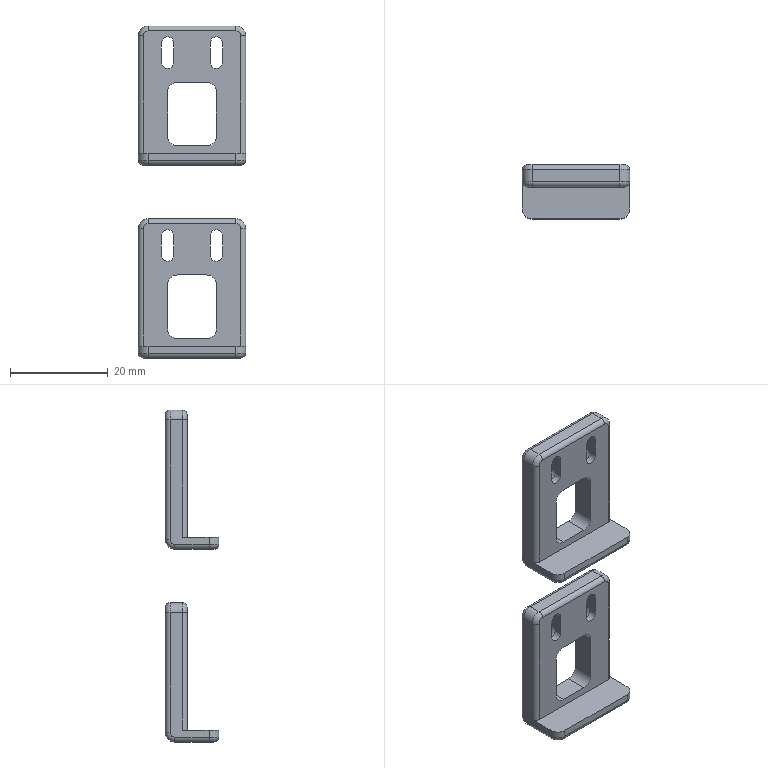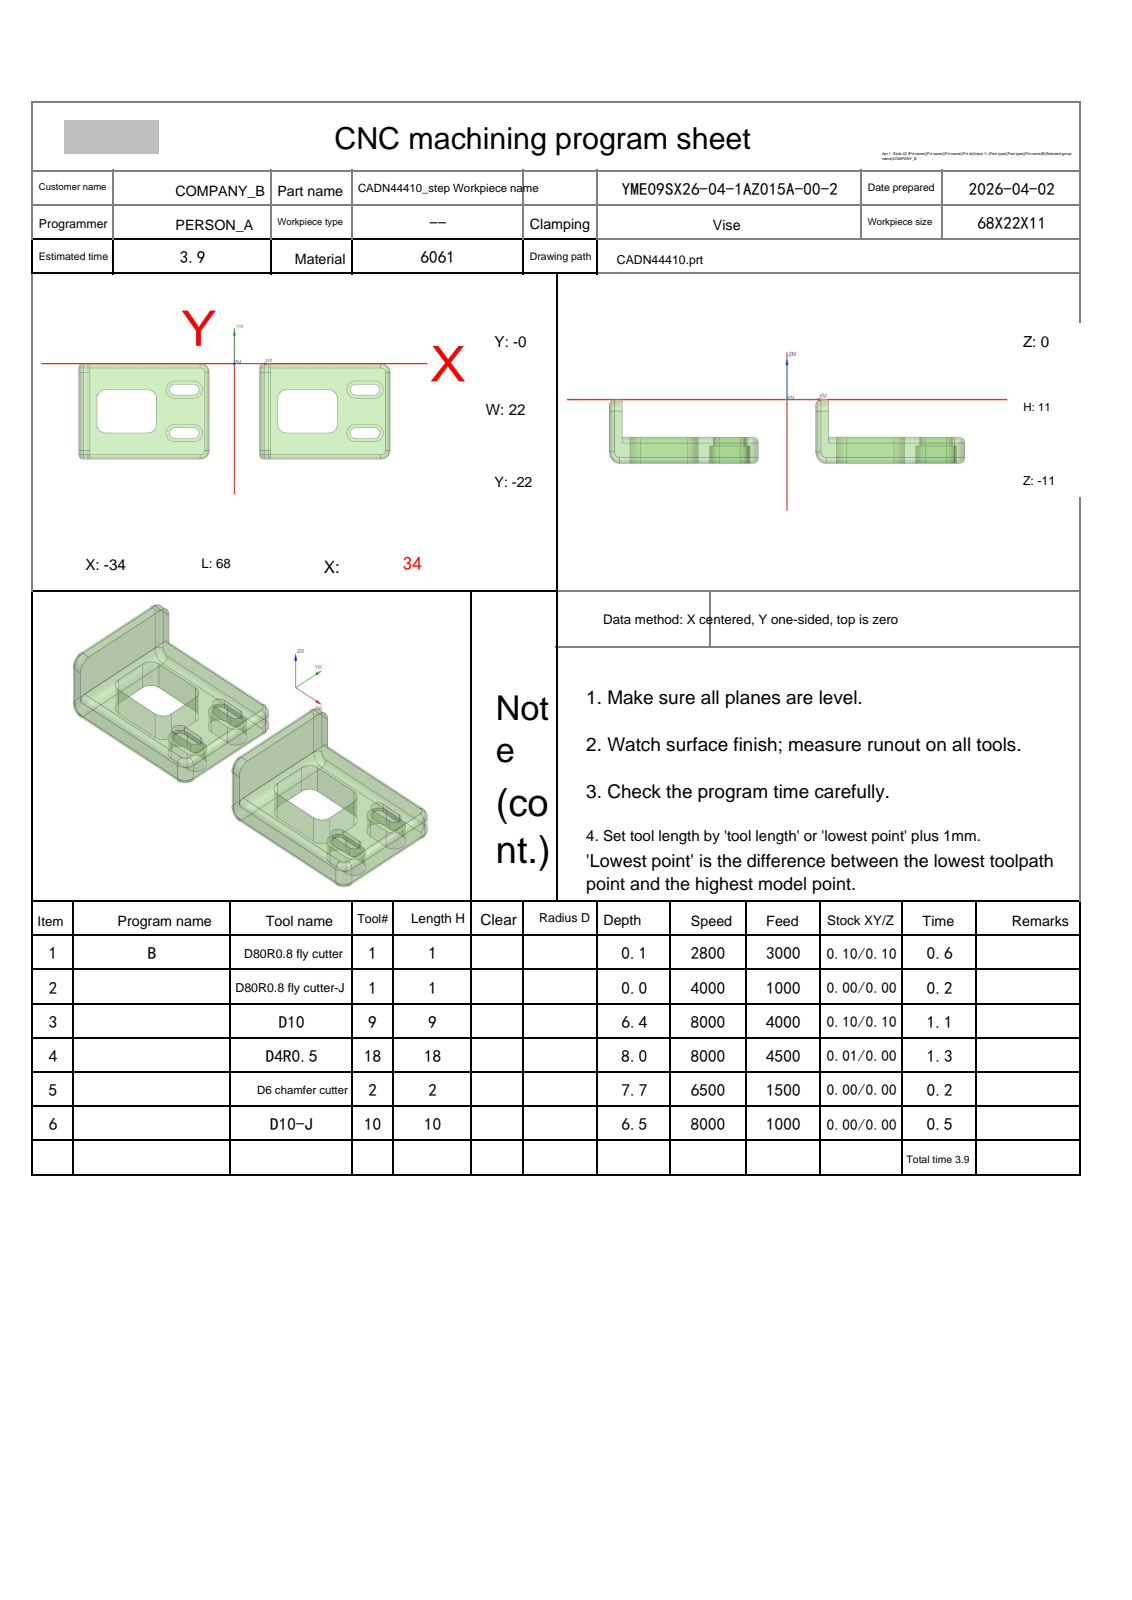NC program | NX | posted by the shop | part box 22 x 11 x 68 mm
Lines 1004 to 3177 of 3177, first 1883 of 2174 lines:
N4 T18 M06
(D4R0.5  D=4. R=0.5 H=18 ce=0.01 di=0.00)
G00 G90 G54 X10.993 Y-22.925 M03 S8000
G43 H18 Z13.5
M08
Z.492
G01 Z-.008 F4500.
G03 X9.085 Y-21.526 I-1.908 J-.601
G01 X9.051
X6.54 Y-21.569
X6.513
G02 X4.908 Y-19.966 I0.0 J1.605
G01 X4.907 Y-18.902
X4.904 Y-18.889
X4.822 Z-.018
X4.872 Y-20.297
X4.898 Y-20.442
G03 X6.303 Y-21.71 I1.784 J.565
G01 X6.584 Y-21.718
X9.051 Y-21.68
Y-21.835 Z-.032
X6.488 Y-21.847
X6.48
G02 X4.738 Y-20.16 I0.0 J1.742
G01 X4.698 Y-18.889
X4.643 Z-.041
X4.638 Z-.05
X4.651 Y-20.015
Y-20.019
G03 X6.584 Y-21.955 I1.937 J0.0
G01 X9.051 Y-21.928
X9.05 Y-22.038 Z-.061
Y-22.069 Z-.072
X6.584 Y-22.085
X6.539
G02 X4.626 Y-20.579 I0.0 J1.968
G01 X4.565 Y-20.297
X4.532 Y-18.889
X4.494 Z-.085
X4.458 Z-.097
X4.487 Y-20.297
X4.528 Y-20.51
G03 X6.559 Y-22.183 I2.03 J.395
G01 X6.572
X9.05 Y-22.168
Y-22.236 Z-.112
Y-22.277 Z-.127
X6.586 Y-22.288
X6.576
G02 X4.415 Y-20.174 I0.0 J2.162
G01 X4.386 Y-18.889
X4.35 Z-.144
X4.316 Z-.16
X4.336 Y-20.227
X4.35 Y-20.368
G03 X6.553 Y-22.375 I2.229 J.234
G01 X6.584
X9.05 Y-22.365
Y-22.424 Z-.179
Y-22.463 Z-.197
X6.303 Y-22.471
G02 X4.273 Y-20.297 I.329 J2.342
G01 X4.246 Y-18.889
X4.212 Z-.218
X4.179 Z-.238
X4.198 Y-20.297
X4.245 Y-20.579
G03 X6.303 Y-22.561 I2.377 J.409
G01 X6.584 Y-22.571
X9.05 Y-22.565
Y-22.608 Z-.26
Y-22.647 Z-.282
X6.584 Y-22.653
X6.303 Y-22.643
G02 X4.175 Y-20.579 I.31 J2.449
X4.098 Y-19.424 I8.609 J1.155
X4.114 Y-18.889 I8.686 J0.0
G01 X4.082 Z-.306
X4.051 Z-.33
X4.054 Y-20.057
X4.075 Y-20.297
G03 X4.575 Y-21.706 I2.879 J.229
X6.542 Y-22.742 I1.967 J1.349
G01 X6.584
X9.05 Y-22.735
Y-22.783 Z-.356
Y-22.829 Z-.382
X6.584 Y-22.836
X6.303 Y-22.825
G02 X4.054 Y-20.599 I.329 J2.581
X3.98 Y-19.35 I10.496 J1.25
X3.99 Y-18.889 I10.57 J0.0
G01 X3.961 Z-.409
X3.932 Z-.436
X3.934 Y-18.902
X3.933 Y-20.015
G03 X4.393 Y-21.686 I3.41 J.041
X6.516 Y-22.909 I2.123 J1.232
G01 X6.519
X8.833 Y-22.906
X9.05 Y-22.905
Y-22.953 Z-.465
Y-22.983 Z-.495
X6.511 Y-22.986
X6.509
G02 X4.258 Y-21.565 I0.0 J2.494
G01 X4.191 Y-21.424
G02 X3.881 Y-20.036 I2.954 J1.388
G01 Y-20.015
Y-18.902
X3.877 Y-18.889
X3.85 Z-.525
X3.825 Z-.556
G03 X3.818 Y-19.371 I17.493 J-.482
X3.842 Y-20.297 I17.499 J0.0
X4.336 Y-21.834 I3.321 J.217
X6.536 Y-23.075 I2.201 J1.331
G01 X6.584
X9.05 Y-23.066
Y-23.109 Z-.588
Y-23.147 Z-.62
X6.584 Y-23.154
X6.543
G02 X4.336 Y-21.951 I0.0 J2.628
X3.823 Y-20.579 I2.737 J1.805
X3.76 Y-19.45 I10.068 J1.128
X3.775 Y-18.889 I10.131 J0.0
G01 X3.752 Z-.654
X3.729 Z-.687
X3.731 Y-20.015
Y-20.023
G03 X4.123 Y-21.706 I3.808 J0.0
X6.559 Y-23.229 I2.436 J1.187
G01 X6.584
X9.05 Y-23.223
Y-23.259 Z-.722
Y-23.294 Z-.757
X6.584 Y-23.299
X6.537 Y-23.3
G02 X4.417 Y-22.269 I0.0 J2.697
X3.732 Y-20.579 I2.635 J2.052
G01 X3.688 Y-20.015
Y-18.902
X3.687 Y-18.889
X3.667 Z-.794
X3.648 Z-.83
X3.649 Y-19.898
G03 X3.734 Y-20.855 I5.559 J.008
X4.336 Y-22.258 I3.286 J.579
X6.533 Y-23.369 I2.198 J1.618
G01 X6.584
X9.05 Y-23.362
Y-23.395 Z-.868
Y-23.427 Z-.906
X6.584 Y-23.432
X6.537 Y-23.433
G02 X4.096 Y-21.988 I0.0 J2.783
X3.651 Y-20.579 I3.187 J1.782
X3.602 Y-19.433 I13.332 J1.146
X3.613 Y-18.889 I13.381 J0.0
G01 X3.596 Z-.945
X3.582 Z-.984
G03 X3.572 Y-19.416 I14.924 J-.528
X3.618 Y-20.579 I14.934 J0.0
X4.054 Y-22.013 I3.744 J.357
X6.531 Y-23.493 I2.476 J1.332
G01 X6.584
X9.05 Y-23.488
Y-23.52 Z-1.025
Y-23.55 Z-1.065
X6.584 Y-23.552
X6.525 Y-23.553
G02 X4.34 Y-22.516 I0.0 J2.819
X3.756 Y-21.419 I2.487 J2.029
X3.568 Y-20.297 I4.243 J1.288
X3.551 Y-19.321 I28.286 J.976
X3.555 Y-18.889 I28.302 J0.0
G01 X3.543 Z-1.106
X3.532 Z-1.148
G03 X3.526 Y-19.374 I20.107 J-.486
X3.562 Y-20.579 I20.113 J0.0
X4.054 Y-22.184 I3.705 J.258
X6.303 Y-23.603 I2.478 J1.438
X8.905 Y-23.61 I2.601 J488.547
G01 X9.05 Y-23.609
Y-23.633 Z-1.191
Y-23.657 Z-1.233
X6.584 Y-23.662
X6.527
G02 X4.054 Y-22.264 I0.0 J2.886
X3.773 Y-21.684 I2.172 J1.411
X3.523 Y-20.297 I4.198 J1.474
G01 X3.514 Y-18.889
X3.501 Z-1.32
X3.506 Y-18.902
X3.512 Y-20.297
Y-20.321
G03 X3.862 Y-21.988 I4.148 J0.0
X6.303 Y-23.702 I2.673 J1.211
G01 X6.584 Y-23.709
X9.05 Y-23.703
Y-23.729 Z-1.365
Y-23.748 Z-1.41
X6.584 Y-23.753
X6.511 Y-23.754
G02 X4.054 Y-22.402 I0.0 J2.908
X3.513 Y-20.579 I3.05 J1.898
G01 X3.501 Y-20.297
X3.493 Y-18.889
X3.49 Y-18.897 Z-1.5
X3.492 Y-20.297
X3.494 Y-20.501
G03 X3.638 Y-21.516 I4.059 J.058
G01 X3.66 Y-21.597
G03 X4.122 Y-22.551 I2.806 J.768
G01 X4.336 Y-22.832
G03 X6.534 Y-23.799 I2.199 J2.016
G01 X6.584
X9.05 Y-23.794
Y-23.814 Z-1.547
Y-23.833 Z-1.593
X6.584 Y-23.837
X6.534 Y-23.838
G02 X3.771 Y-21.988 I0.0 J2.989
X3.492 Y-20.559 I3.55 J1.434
G01 X3.49 Y-20.297
Y-18.897
Z-1.687
Y-20.579
X3.492 Y-20.697
G03 X3.773 Y-22.045 I3.567 J.04
X6.52 Y-23.872 I2.746 J1.151
G01 X6.584 Y-23.871
X9.05 Y-23.865
Y-23.881 Z-1.734
Y-23.895 Z-1.782
X6.584 Y-23.901
X6.515 Y-23.902
G02 X3.773 Y-22.097 I0.0 J2.985
X3.492 Y-20.798 I3.125 J1.356
G01 X3.49 Y-20.579
Y-18.897
Z-1.878
Y-20.579
X3.492 Y-20.861
G03 X3.618 Y-21.706 I3.095 J.03
X6.514 Y-23.927 I2.896 J.777
G01 X6.584
X9.05 Y-23.918
Y-23.933 Z-1.927
Y-23.941 Z-1.976
X6.584 Y-23.952
X6.519 Y-23.953
G02 X3.773 Y-22.181 I0.0 J3.013
X3.49 Y-20.861 I2.962 J1.326
G01 Y-18.897
Z-2.074
Y-20.915
G03 X3.773 Y-22.212 I3.114 J0.0
X6.517 Y-23.973 I2.744 J1.258
G01 X6.584 Y-23.972
X9.046 Y-23.964
X9.033 Y-23.984 Z-2.173
X8.833 Y-23.985
X6.584 Y-23.987
X6.375 Y-23.984
G02 X5.098 Y-23.626 I.091 J2.779
X4.299 Y-23.015 I1.142 J2.32
X3.946 Y-22.551 I1.794 J1.734
X3.489 Y-20.916 I2.7 J1.635
G01 X3.49 Y-20.861
Y-18.897
Z-2.255
Y-20.861
X3.492 Y-21.063
G03 X4.283 Y-23.013 I3.087 J.116
X5.134 Y-23.66 I2.183 J1.99
X6.489 Y-23.993 I1.354 J2.585
G01 X6.491
X9.021 Y-23.991
X9.01 Y-23.998 Z-2.336
X8.833
X6.584 Y-23.999
X6.51 Y-24.
G02 X3.492 Y-21.081 I0.0 J3.019
G01 X3.49 Y-20.861
Y-18.897
Z-2.418
Y-20.861
X3.491 Y-21.02
G03 X6.506 Y-24.005 I3.015 J.03
G01 X6.507
X8.998 Y-24.004
X8.987 Y-24.009 Z-2.5
X6.504 Y-24.01
X6.503
G02 X3.491 Y-21.026 I0.0 J3.011
G01 X3.49 Y-20.861
Y-18.897
G00 Z13.5
X2.904 Y-5.06
Z.492
G01 Z-.008
G03 X4.904 Y-3.111 I0.0 J2.
G01 X4.933 Y-1.959
G02 X6.51 Y-.423 I1.577 J-.04
G01 X6.594 Y-.425
X9.055 Y-.557
G00 Z.482
X11.089 Y1.002
G01 Z-.018
G02 X9.194 Y-.359 I-1.895 J.64
G01 X9.052 Y-.353
G03 X7.028 Y-.281 I-2.023 J-28.265
X6.303 Y-.29 I0.0 J-28.338
X4.898 Y-1.558 I.379 J-1.833
G01 X4.872 Y-1.703
X4.822 Y-3.111
X4.719 Z-.025
X4.698 Z-.032
X4.758 Y-1.794
G02 X6.491 Y-.139 I1.733 J-.08
G01 X6.512
X9.051 Y-.17
Y-.077 Z-.05
X6.576 Y-.044
X6.551
G03 X4.684 Y-1.847 I0.0 J-1.869
G01 X4.638 Y-3.111
X4.568 Z-.061
X4.532 Z-.072
X4.561 Y-1.851
G02 X6.541 Y.083 I1.979 J-.046
G01 X6.552
X9.05 Y.069
Y.136 Z-.085
Y.17 Z-.097
X6.584 Y.185
X6.522 Y.184
G03 X4.53 Y-1.481 I.029 J-2.058
G01 X4.487 Y-1.703
X4.458 Y-3.111
X4.421 Z-.112
X4.386 Z-.127
X4.415 Y-1.825
G02 X6.508 Y.286 I2.16 J-.048
G01 X6.584 Y.289
X9.05 Y.282
Y.333 Z-.144
Y.379 Z-.16
X8.552 Y.365
X6.569 Y.374
X6.559
G03 X4.383 Y-1.465 I0.0 J-2.207
X4.292 Y-2.554 I6.447 J-1.089
X4.316 Y-3.111 I6.538 J0.0
G01 X4.28 Z-.179
X4.246 Z-.197
G02 X4.223 Y-2.561 I6.502 J.55
X4.331 Y-1.38 I6.525 J0.0
X6.546 Y.466 I2.217 J-.408
G01 X9.05 Y.468
Y.514 Z-.218
Y.557 Z-.238
X6.584 Y.568
X6.303 Y.557
G03 X4.245 Y-1.421 I.308 J-2.38
G01 X4.198 Y-1.703
X4.179 Y-3.111
X4.146 Z-.26
X4.114 Z-.282
G02 X4.098 Y-2.576 I8.669 J.536
X4.175 Y-1.421 I8.686 J0.0
X6.303 Y.649 I2.449 J-.389
G01 X9.05 Y.639
Y.693 Z-.306
Y.728 Z-.33
X6.538 Y.748
X6.52
G03 X5.179 Y.309 I0.0 J-2.27
X4.075 Y-1.703 I1.603 J-2.188
G01 X4.054 Y-1.943
X4.051 Y-3.111
X4.02 Z-.356
X3.99 Z-.382
G02 X3.988 Y-2.793 I23.526 J.319
X4.014 Y-1.703 I23.528 J0.0
X5.46 Y.582 I2.765 J-.15
X6.575 Y.834 I1.115 J-2.337
G01 X6.584
X9.05 Y.824
Y.869 Z-.409
Y.907 Z-.436
X6.443 Y.906
G03 X4.857 Y.258 I0.0 J-2.266
X3.947 Y-1.798 I2.13 J-2.172
X3.929 Y-2.736 I24.567 J-.938
X3.932 Y-3.111 I24.585 J0.0
G01 X3.904 Z-.465
X3.877 Z-.495
G02 X3.863 Y-2.571 I10.135 J.54
X3.916 Y-1.529 I10.149 J0.0
X5.097 Y.551 I2.961 J-.306
X6.303 Y.991 I1.492 J-2.219
G01 X9.05 Y.988
Y1.029 Z-.525
Y1.061 Z-.556
X6.584 Y1.076
X6.531
G03 X4.653 Y.251 I0.0 J-2.55
X3.866 Y-1.501 I2.242 J-2.059
X3.812 Y-2.584 I10.681 J-1.084
X3.825 Y-3.111 I10.736 J0.0
G01 X3.799 Z-.588
X3.775 Z-.62
G02 X3.76 Y-2.55 I10.115 J.562
X3.823 Y-1.421 I10.131 J0.0
X4.576 Y.269 I3.216 J-.419
X6.546 Y1.155 I1.97 J-1.749
G01 X6.584
X9.05 Y1.136
Y1.175 Z-.654
Y1.212 Z-.687
X6.584 Y1.229
X6.559
G03 X4.123 Y-.294 I0.0 J-2.71
X3.731 Y-1.977 I3.416 J-1.683
G01 Y-1.985
X3.735 Y-3.098
X3.729 Y-3.111
X3.687 Z-.757
X3.694 Y-3.098
X3.688 Y-1.985
X3.732 Y-1.421
G02 X4.417 Y.269 I3.321 J-.362
X6.535 Y1.299 I2.118 J-1.663
G01 X6.584 Y1.298
X9.05 Y1.284
Y1.32 Z-.794
Y1.351 Z-.83
X6.584 Y1.367
X6.535
G03 X4.153 Y-.012 I0.0 J-2.746
X3.665 Y-1.703 I3.224 J-1.848
X3.644 Y-2.697 I24.386 J-.994
X3.648 Y-3.111 I24.406 J0.0
G01 X3.63 Z-.868
X3.613 Z-.906
G02 X3.602 Y-2.567 I13.37 J.544
X3.651 Y-1.421 I13.381 J0.0
X4.096 Y-.012 I3.632 J-.373
X6.534 Y1.432 I2.438 J-1.336
G01 X6.584 Y1.431
X9.05 Y1.419
Y1.456 Z-.945
Y1.484 Z-.984
X6.584 Y1.494
X6.534
G03 X4.054 Y.013 I0.0 J-2.817
X3.618 Y-1.421 I3.307 J-1.791
X3.572 Y-2.584 I14.888 J-1.163
X3.582 Y-3.111 I14.934 J0.0
G01 X3.567 Z-1.025
X3.555 Z-1.065
G02 X3.551 Y-2.679 I28.299 J.433
X3.568 Y-1.703 I28.302 J0.0
X3.854 Y-.294 I4.431 J-.166
X4.336 Y.51 I3.222 J-1.384
X6.533 Y1.555 I2.197 J-1.787
G01 X6.584 Y1.554
X9.05 Y1.548
Y1.578 Z-1.106
Y1.601 Z-1.148
X6.584 Y1.608
X6.522
G03 X4.054 Y.184 I0.0 J-2.85
X3.562 Y-1.421 I3.213 J-1.863
X3.526 Y-2.626 I20.077 J-1.205
X3.532 Y-3.111 I20.113 J0.0
G01 X3.522 Z-1.191
X3.514 Z-1.233
X3.523 Y-1.703
G02 X3.773 Y-.316 I4.448 J-.087
X5.306 Y1.396 I2.847 J-1.006
X6.543 Y1.663 I1.237 J-2.74
G01 X6.584 Y1.662
X9.05 Y1.655
Y1.681 Z-1.277
Y1.703 Z-1.32
X6.584 Y1.709
X6.519 Y1.71
G03 X5.46 Y1.511 I0.0 J-2.925
X3.773 Y-.229 I1.111 J-2.764
X3.512 Y-1.683 I3.919 J-1.454
G01 Y-1.703
X3.506 Y-3.098
X3.501 Y-3.111
X3.493 Z-1.41
X3.501 Y-1.703
X3.513 Y-1.421
G02 X4.054 Y.402 I3.592 J-.075
X6.512 Y1.754 I2.458 J-1.558
G01 X6.584 Y1.753
X9.05 Y1.748
Y1.774 Z-1.455
Y1.793 Z-1.5
X6.584 Y1.799
X6.536
G03 X4.336 Y.832 I0.0 J-2.986
X3.69 Y-.294 I2.517 J-2.19
X3.494 Y-1.518 I4.102 J-1.285
G01 X3.492 Y-1.703
X3.49 Y-3.111
Z-1.593
X3.492 Y-1.441
X3.507 Y-1.139
G02 X4.336 Y.879 I3.333 J-.189
X6.54 Y1.838 I2.204 J-2.053
G01 X6.584
X9.05 Y1.832
Y1.85 Z-1.64
Y1.862 Z-1.687
X6.584 Y1.872
X6.523
G03 X4.054 Y.565 I0.0 J-2.984
X3.502 Y-1.139 I2.793 J-1.848
G01 X3.492 Y-1.303
X3.49 Y-3.111
Z-1.782
X3.492 Y-1.202
X3.503 Y-1.02
G02 X4.05 Y.602 I3.263 J-.197
X6.517 Y1.902 I2.467 J-1.689
G01 X6.584
X9.05 Y1.891
Y1.906 Z-1.83
Y1.916 Z-1.878
G03 X6.584 Y1.927 I-3.097 J-399.102
G01 X6.516 Y1.928
G03 X4.331 Y.987 I0.0 J-3.006
X3.492 Y-1.118 I2.351 J-2.157
G01 X3.49 Y-1.421
Y-3.111
Z-1.976
Y-1.139
X3.492 Y-1.056
G02 X4.768 Y1.396 I3.101 J-.054
X6.53 Y1.953 I1.763 J-2.509
G01 X6.584
G02 X9.05 Y1.94 I-.437 J-322.397
G01 X9.048 Y1.955 Z-2.025
X9.046 Y1.963 Z-2.074
X6.584 Y1.971
X6.523 Y1.972
G03 X4.767 Y1.417 I0.0 J-3.056
X3.492 Y-1. I1.804 J-2.495
G01 X3.49 Y-1.139
Y-3.111
Z-2.173
Y-1.139
X3.491 Y-1.036
G02 X3.997 Y.637 I3.154 J-.041
X4.76 Y1.426 I2.577 J-1.731
X5.952 Y1.936 I1.819 J-2.603
G01 X6.022 Y1.947
X6.447 Y1.986
X9.033 Y1.982
X9.021 Y1.99 Z-2.255
G03 X7.576 Y1.994 I-1.445 J-259.203
X6.584 Y1.992 I0.0 J-259.207
G01 X6.499 Y1.995
X6.4 Y2.003
X6.303 Y1.98
X6.022 Y1.959
X5.982 Y1.947
X5.951 Y1.944
X5.858 Y1.926
X5.741 Y1.892
G03 X3.773 Y.246 I.761 J-2.909
G01 X3.671 Y-.012
X3.587 Y-.294
X3.528 Y-.576
X3.497 Y-.858
X3.492 Y-.937
X3.49 Y-3.111
Z-2.336
X3.492 Y-.919
X3.496 Y-.858
G02 X6.508 Y2. I3.012 J-.159
G01 X6.584 Y1.999
X9.01 Y1.997
X8.998 Y2.004 Z-2.418
X6.509 Y2.005
X6.508
G03 X3.496 Y-.84 I0.0 J-3.017
G01 X3.492 Y-.901
X3.49 Y-3.111
Z-2.5
Y-1.139
X3.491 Y-.973
G02 X6.491 Y2.009 I3.01 J-.028
G01 X6.584 Y2.01
X8.987 Y2.009
G00 Z13.5
X-28.574 Y-22.959
Z.492
G01 Z-.008
G03 X-30.449 Y-21.527 I-1.918 J-.568
G01 X-33.6 Y-21.461
G02 X-34.582 Y-20.015 I.665 J1.509
G01 Y-18.902
X-34.597 Y-18.889
X-34.678 Z-.018
X-34.616 Y-20.297
X-34.573 Y-20.554
G03 X-33.172 Y-21.712 I1.765 J.708
G01 X-30.449 Y-21.68
Y-21.835 Z-.032
X-30.93
X-32.945 Y-21.861
X-32.968
G02 X-34.771 Y-20.105 I0.0 J1.803
G01 X-34.803 Y-18.889
X-34.857 Z-.041
X-34.862 Z-.05
G03 X-34.891 Y-19.446 I5.405 J-.558
X-34.823 Y-20.297 I5.433 J0.0
X-32.918 Y-21.956 I1.906 J.265
G01 X-32.892
X-30.449 Y-21.928
X-30.45 Y-22.038 Z-.061
Y-22.069 Z-.072
X-32.947 Y-22.085
X-32.959
G02 X-34.926 Y-20.18 I0.0 J1.968
G01 X-34.968 Y-18.889
X-35.006 Z-.085
X-35.042 Z-.097
G03 X-35.072 Y-19.43 I4.795 J-.541
X-34.897 Y-20.718 I4.825 J0.0
X-32.97 Y-22.184 I1.927 J.534
G01 X-32.957
X-30.45 Y-22.167
Y-22.237 Z-.112
Y-22.277 Z-.127
X-32.925 Y-22.288
X-32.935
G02 X-35.021 Y-20.592 I0.0 J2.131
X-35.141 Y-19.438 I5.526 J1.154
X-35.114 Y-18.889 I5.645 J0.0
G01 X-35.15 Z-.144
X-35.185 Z-.16
X-35.159 Y-20.186
G03 X-32.927 Y-22.374 I2.232 J.044
G01 X-32.919
X-30.45 Y-22.365
Y-22.424 Z-.179
Y-22.463 Z-.197
X-32.907 Y-22.473
X-32.916
G02 X-35.23 Y-20.202 I0.0 J2.314
G01 X-35.254 Y-18.889
X-35.321 Z-.238
X-35.317 Y-18.902
Y-20.015
G03 X-34.927 Y-21.424 I2.825 J.024
X-32.939 Y-22.572 I1.988 J1.148
G01 X-32.892 Y-22.571
X-30.45 Y-22.565
Y-22.608 Z-.26
Y-22.646 Z-.282
X-32.892 Y-22.653
X-33.172 Y-22.645
G02 X-35.322 Y-20.579 I.272 J2.434
X-35.405 Y-19.436 I7.785 J1.143
X-35.386 Y-18.889 I7.868 J0.0
G01 X-35.418 Z-.306
X-35.449 Z-.33
G03 X-35.465 Y-19.427 I9.052 J-.538
X-35.414 Y-20.388 I9.068 J0.0
X-34.919 Y-21.706 I2.706 J.264
G01 X-34.853 Y-21.797
G03 X-32.966 Y-22.743 I1.888 J1.41
G01 X-32.892 Y-22.742
X-30.45 Y-22.735
Y-22.783 Z-.356
Y-22.829 Z-.382
X-30.93 Y-22.832
X-32.892 Y-22.836
X-33.172 Y-22.828
G02 X-35.414 Y-20.743 I.291 J2.561
X-35.527 Y-19.415 I7.732 J1.329
X-35.51 Y-18.889 I7.845 J0.0
G01 X-35.539 Z-.409
X-35.568 Z-.436
X-35.566 Y-18.902
X-35.567 Y-20.015
G03 X-35.24 Y-21.424 I3.272 J.017
G01 X-35.195 Y-21.518
G03 X-32.977 Y-22.911 I2.218 J1.068
G01 X-32.971
X-30.45 Y-22.904
Y-22.953 Z-.465
Y-22.983 Z-.495
X-30.65 Y-22.985
X-32.892 Y-22.991
X-32.993 Y-22.99
G02 X-35.159 Y-21.726 I.023 J2.526
X-35.623 Y-20.015 I3.006 J1.733
G01 X-35.618 Y-18.902
X-35.623 Y-18.889
X-35.65 Z-.525
X-35.675 Z-.556
G03 X-35.68 Y-19.305 I21.399 J-.416
X-35.656 Y-20.297 I21.404 J0.0
X-35.134 Y-21.885 I3.3 J.207
X-32.956 Y-23.076 I2.178 J1.395
G01 X-32.892 Y-23.075
X-30.45 Y-23.066
Y-23.109 Z-.588
Y-23.147 Z-.62
X-32.961 Y-23.154
X-32.969
G02 X-35.191 Y-21.912 I0.0 J2.61
X-35.723 Y-20.032 I3.056 J1.88
G01 Y-20.015
X-35.725 Y-18.889
X-35.748 Z-.654
X-35.771 Z-.687
X-35.77 Y-20.015
Y-20.021
G03 X-35.378 Y-21.706 I3.815 J0.0
X-32.94 Y-23.229 I2.438 J1.188
G01 X-32.892
X-30.65 Y-23.224
X-30.45 Y-23.222
Y-23.259 Z-.722
Y-23.294 Z-.757
X-32.892 Y-23.299
X-32.958 Y-23.3
G02 X-35.285 Y-21.988 I0.0 J2.719
X-35.812 Y-20.049 I3.308 J1.939
G01 Y-20.015
Y-18.902
X-35.813 Y-18.889
X-35.833 Z-.794
X-35.852 Z-.83
G03 X-35.865 Y-19.439 I11.982 J-.551
X-35.811 Y-20.579 I11.995 J0.0
X-35.346 Y-21.988 I3.601 J.407
X-32.956 Y-23.369 I2.39 J1.375
G01 X-32.892
X-30.45 Y-23.362
Y-23.395 Z-.868
Y-23.427 Z-.906
X-32.981 Y-23.432
X-32.987
G02 X-35.098 Y-22.431 I0.0 J2.726
X-35.746 Y-21.13 I2.545 J2.079
X-35.885 Y-20.015 I4.784 J1.165
G01 Y-18.902
X-35.887 Y-18.889
X-35.904 Z-.945
X-35.919 Z-.984
X-35.916 Y-18.902
X-35.915 Y-20.015
Y-20.04
G03 X-35.781 Y-21.142 I4.596 J0.0
G01 X-35.739 Y-21.301
G03 X-34.999 Y-22.616 I2.938 J.787
G01 X-34.961 Y-22.656
G03 X-33.085 Y-23.487 I1.949 J1.863
G01 X-32.892 Y-23.493
X-30.45 Y-23.488
Y-23.52 Z-1.025
Y-23.549 Z-1.065
X-30.65 Y-23.551
X-32.959 Y-23.552
X-32.961
G02 X-35.357 Y-22.247 I0.0 J2.852
X-35.808 Y-21.188 I2.848 J1.839
X-35.939 Y-20.062 I4.767 J1.126
G01 Y-20.015
X-35.941 Y-18.902
X-35.946 Y-18.889
X-35.957 Z-1.106
X-35.968 Z-1.148
G03 X-35.969 Y-19.208 I50.531 J-.32
X-35.957 Y-20.297 I50.532 J0.0
X-35.559 Y-21.988 I4.179 J.093
X-33.172 Y-23.605 I2.614 J1.288
G01 X-30.45 Y-23.609
Y-23.633 Z-1.191
Y-23.656 Z-1.233
X-32.892 Y-23.662
X-32.971 Y-23.663
G02 X-35.414 Y-22.315 I0.0 J2.888
X-35.879 Y-21.142 I2.826 J1.799
X-35.984 Y-20.052 I5.586 J1.09
G01 Y-20.015
X-35.982 Y-18.906
X-35.986 Y-18.889
X-35.999 Z-1.32
X-35.992 Y-18.906
G03 X-35.995 Y-19.434 I42.706 J-.528
X-35.98 Y-20.579 I42.709 J0.0
G01 X-35.974 Y-20.665
X-35.919 Y-21.049
G03 X-35.171 Y-22.705 I3.236 J.465
X-32.996 Y-23.709 I2.175 J1.854
G01 X-32.988
X-30.45 Y-23.702
Y-23.729 Z-1.365
Y-23.747 Z-1.41
X-32.892 Y-23.753
X-33.172 Y-23.751
G02 X-35.518 Y-22.282 I.201 J2.929
X-35.993 Y-20.579 I3.25 J1.824
X-36.007 Y-18.978 I87.938 J1.601
G01 Y-18.889
X-36.01 Y-18.897 Z-1.5
X-36.007 Y-20.297
X-35.999 Y-20.579
G03 X-35.7 Y-21.988 I3.673 J.044
X-32.968 Y-23.8 I2.732 J1.154
G01 X-32.892 Y-23.799
X-30.45 Y-23.793
Y-23.814 Z-1.547
Y-23.833 Z-1.593
X-32.892 Y-23.837
X-32.943 Y-23.838
G02 X-34.293 Y-23.535 I0.0 J3.164
G01 X-34.312 Y-23.517
X-34.393 Y-23.474
G02 X-35.849 Y-21.643 I1.436 J2.637
G01 X-35.869 Y-21.572
G02 X-36.006 Y-20.579 I3.616 J1.003
G01 X-36.01 Y-20.297
Y-18.897
Z-1.687
Y-20.579
Y-20.628
G03 X-35.694 Y-22.12 I3.68 J0.0
X-33.172 Y-23.864 I2.711 J1.225
G01 X-32.892 Y-23.871
X-30.45 Y-23.865
Y-23.882 Z-1.734
Y-23.895 Z-1.782
X-32.892 Y-23.901
X-33.055 Y-23.898
G02 X-35.664 Y-22.23 I.058 J2.964
G01 X-35.694 Y-22.168
G02 X-36.003 Y-20.861 I2.944 J1.385
G01 X-36.01 Y-20.579
Y-18.897
Z-1.878
Y-20.579
X-36.007 Y-20.861
G03 X-35.694 Y-22.21 I3.254 J.044
X-33.172 Y-23.922 I2.703 J1.269
G01 X-32.892 Y-23.927
X-30.45 Y-23.918
Y-23.933 Z-1.927
Y-23.941 Z-1.976
X-32.892 Y-23.952
X-32.974 Y-23.954
G02 X-35.993 Y-21.146 I0.0 J3.028
X-36.01 Y-20.687 I6.299 J.46
G01 Y-18.897
Z-2.074
X-36.009 Y-20.716
G03 X-35.996 Y-21.138 I6.89 J.003
X-32.982 Y-23.972 I3.015 J.186
G01 X-32.971
X-30.453 Y-23.964
X-30.466 Y-23.983 Z-2.173
X-30.65 Y-23.985
X-32.982 Y-23.987
X-32.984
G02 X-36. Y-21.116 I0.0 J3.019
X-36.009 Y-20.727 I7.951 J.392
G01 X-36.01 Y-18.897
Z-2.255
Y-20.861
X-36.001 Y-21.142
G03 X-33.137 Y-23.989 I3.008 J.162
G01 X-32.892 Y-23.993
X-30.65 Y-23.991
X-30.476 Y-23.99
X-30.487 Y-23.997 Z-2.336
X-30.65 Y-23.998
X-32.892 Y-23.999
X-33.137 Y-23.996
G02 X-36.003 Y-21.142 I.14 J3.007
G01 X-36.01 Y-20.861
Y-18.897
Z-2.418
Y-20.994
G03 X-32.999 Y-24.005 I3.011 J0.0
G01 X-30.65
X-30.497 Y-24.004
X-30.508 Y-24.009 Z-2.5
X-32.892 Y-24.01
X-33.155 Y-24.006
G02 X-33.416 Y-23.981 I.155 J3.006
G01 X-33.548 Y-23.96
G02 X-34.374 Y-23.678 I.563 J3.003
X-34.764 Y-23.439 I1.352 J2.642
X-35.021 Y-23.23 I1.764 J2.439
G01 X-35.224 Y-23.029
G02 X-35.419 Y-22.792 I2.224 J2.029
X-35.974 Y-21.514 I2.531 J1.861
G01 Y-21.457
X-36.006 Y-21.142
X-36.01 Y-20.861
Y-18.897
G00 Z13.5
X-36.597 Y-4.306
Z.492
G01 Z-.008
X-36.431 Y-4.313
G03 X-34.597 Y-3.111 I0.0 J2.
G01 X-34.592 Y-3.098
Y-2.058
G02 X-32.948 Y-.414 I1.644 J0.0
G01 X-32.856 Y-.416
X-30.444 Y-.552
G00 Z.482
X-28.414 Y1.001
G01 Z-.018
G02 X-30.308 Y-.357 I-1.894 J.642
G01 X-30.448 Y-.352
G03 X-32.489 Y-.28 I-2.04 J-28.99
X-33.172 Y-.288 I0.0 J-29.062
X-34.675 Y-2.074 I.309 J-1.786
G01 Y-2.12
X-34.678 Y-3.111
X-34.781 Z-.025
X-34.803 Z-.032
X-34.745 Y-1.813
G02 X-32.995 Y-.139 I1.75 J-.078
G01 X-32.973
X-30.449 Y-.17
Y-.077 Z-.05
X-32.892 Y-.044
X-32.937
G03 X-34.823 Y-1.703 I0.0 J-1.902
G01 X-34.853 Y-1.901
X-34.862 Y-3.111
X-34.932 Z-.061
X-34.968 Z-.072
X-34.926 Y-1.813
G02 X-32.965 Y.086 I1.961 J-.063
G01 X-32.952
X-30.45 Y.069
Y.136 Z-.085
Y.17 Z-.097
X-32.969 Y.183
X-32.98
G03 X-34.893 Y-1.269 I0.0 J-1.987
X-35.072 Y-2.57 I4.646 J-1.302
X-35.042 Y-3.111 I4.825 J0.0
G01 X-35.079 Z-.112
X-35.114 Z-.127
G02 X-35.141 Y-2.562 I5.619 J.55
X-35.021 Y-1.403 I5.645 J0.0
X-32.984 Y.287 I2.082 J-.437
G01 X-32.892 Y.289
X-30.45 Y.281
Y.335 Z-.144
Y.378 Z-.16
X-30.93 Y.365
X-32.919 Y.377
X-32.932
G03 X-35.124 Y-1.497 I0.0 J-2.219
G01 X-35.157 Y-1.703
X-35.185 Y-3.111
X-35.22 Z-.179
X-35.254 Z-.197
G02 X-35.281 Y-2.55 I5.867 J.562
X-35.145 Y-1.293 I5.894 J0.0
X-32.957 Y.469 I2.188 J-.477
G01 X-30.45 Y.468
Y.516 Z-.218
Y.556 Z-.238
X-32.892 Y.568
X-32.898
G03 X-34.013 Y.315 I0.0 J-2.58
X-35.3 Y-1.859 I1.264 J-2.217
G01 X-35.321 Y-3.111
X-35.354 Z-.26
X-35.386 Z-.282
G02 X-35.405 Y-2.564 I7.849 J.548
X-35.322 Y-1.421 I7.868 J0.0
X-33.172 Y.652 I2.437 J-.376
G01 X-30.45 Y.639
Y.693 Z-.306
Y.728 Z-.33
X-32.892 Y.748
X-32.91
G03 X-34.013 Y.502 I0.0 J-2.597
X-35.385 Y-1.421 I1.231 J-2.33
X-35.467 Y-2.568 I7.95 J-1.147
X-35.449 Y-3.111 I8.032 J0.0
G01 X-35.48 Z-.356
X-35.51 Z-.382
G02 X-35.527 Y-2.585 I7.827 J.526
X-35.414 Y-1.257 I7.845 J0.0
X-33.172 Y.826 I2.528 J-.473
G01 X-32.892 Y.834
X-30.45 Y.824
Y.869 Z-.409
Y.906 Z-.436
X-32.981 Y.908
X-32.983
G03 X-35.091 Y-.288 I0.0 J-2.455
X-35.567 Y-1.985 I2.896 J-1.729
G01 X-35.566 Y-3.098
X-35.568 Y-3.111
X-35.596 Z-.465
X-35.623 Z-.495
G02 X-35.626 Y-2.753 I25.824 J.359
X-35.604 Y-1.703 I25.827 J0.0
X-34.406 Y.551 I3.042 J-.172
X-32.97 Y.993 I1.436 J-2.115
G01 X-32.965
X-30.45 Y.988
Y1.03 Z-.525
Y1.061 Z-.556
X-32.98 Y1.076
X-32.995
G03 X-34.874 Y.221 I0.0 J-2.49
X-35.656 Y-1.703 I2.418 J-2.105
X-35.68 Y-2.695 I21.381 J-.993
X-35.675 Y-3.111 I21.404 J0.0
G01 X-35.701 Z-.588
X-35.725 Z-.62
G02 X-35.726 Y-2.776 I33.351 J.335
X-35.712 Y-1.783 I33.353 J0.0
X-34.923 Y.269 I3.323 J-.099
X-32.951 Y1.155 I1.973 J-1.753
G01 X-32.892
X-30.45 Y1.136
Y1.175 Z-.654
Y1.211 Z-.687
X-32.892 Y1.229
X-32.94
G03 X-35.378 Y-.294 I0.0 J-2.712
X-35.77 Y-1.979 I3.422 J-1.685
G01 Y-1.985
X-35.764 Y-3.098
X-35.771 Y-3.111
X-35.793 Z-.722
X-35.813 Z-.757
G02 X-35.815 Y-2.766 I33.836 J.345
X-35.798 Y-1.703 I33.838 J0.0
X-35.285 Y-.012 I3.651 J-.185
X-32.961 Y1.299 I2.325 J-1.404
G01 X-32.892
X-30.45 Y1.284
Y1.32 Z-.794
Y1.351 Z-.83
X-32.892 Y1.367
X-32.962 Y1.368
G03 X-35.346 Y-.012 I0.0 J-2.748
X-35.811 Y-1.421 I3.137 J-1.816
X-35.865 Y-2.561 I11.941 J-1.14
X-35.852 Y-3.111 I11.995 J0.0
G01 X-35.87 Z-.868
X-35.887 Z-.906
G02 X-35.895 Y-2.582 I17.308 J.53
X-35.873 Y-1.703 I17.316 J0.0
X-35.659 Y-.576 I4.383 J-.249
X-34.688 Y.833 I2.896 J-.957
X-32.978 Y1.433 I1.71 J-2.137
G01 X-32.892 Y1.431
X-30.45 Y1.418
Y1.456 Z-.945
Y1.484 Z-.984
X-32.892 Y1.494
X-32.976 Y1.495
G03 X-34.293 Y1.164 I0.0 J-2.786
X-35.706 Y-.576 I1.489 J-2.652
X-35.915 Y-1.974 I4.558 J-1.398
G01 Y-1.985
X-35.916 Y-3.098
X-35.919 Y-3.111
X-35.933 Z-1.025
X-35.946 Z-1.065
X-35.933 Y-1.782
G02 X-35.708 Y-.467 I4.175 J-.039
X-34.853 Y.841 I3.003 J-1.029
X-32.959 Y1.555 I1.895 J-2.156
G01 X-32.892 Y1.554
X-30.45 Y1.548
Y1.578 Z-1.106
Y1.601 Z-1.148
X-33.017 Y1.608
X-33.024
G03 X-34.06 Y1.396 I0.0 J-2.641
X-35.683 Y-.294 I1.173 J-2.751
X-35.957 Y-1.703 I4.132 J-1.535
G01 X-35.968 Y-3.111
X-35.978 Z-1.191
X-35.986 Z-1.233
X-35.982 Y-3.094
X-35.984 Y-1.985
Y-1.948
G02 X-35.879 Y-.858 I5.691 J0.0
X-35.247 Y.551 I3.263 J-.617
X-32.97 Y1.663 I2.278 J-1.776
G01 X-32.892 Y1.662
X-30.45 Y1.654
Y1.681 Z-1.277
Y1.703 Z-1.32
X-32.892 Y1.709
X-33.172 Y1.704
G03 X-34.742 Y1.114 I.182 J-2.871
X-35.839 Y-.56 I1.969 J-2.487
X-35.984 Y-1.586 I4.252 J-1.126
X-35.995 Y-2.566 I42.698 J-.98
X-35.992 Y-3.094 I42.709 J0.0
G01 X-35.999 Y-3.111
X-36.007 Z-1.41
X-35.997 Y-1.703
X-35.993 Y-1.421
G02 X-35.518 Y.282 I3.725 J-.121
X-33.172 Y1.749 I2.54 J-1.451
G01 X-32.892 Y1.753
X-30.45 Y1.747
Y1.774 Z-1.455
Y1.793 Z-1.5
X-32.892 Y1.799
X-32.968 Y1.8
G03 X-35.694 Y0.0 I0.0 J-2.965
X-35.999 Y-1.421 I3.359 J-1.464
G01 X-36.007 Y-1.703
X-36.01 Y-3.111
Z-1.593
Y-1.703
X-36.006 Y-1.421
G02 X-35.597 Y.269 I3.709 J-.003
X-34.535 Y1.396 I2.67 J-1.452
G01 X-34.312 Y1.517
X-34.296 Y1.532
G02 X-32.947 Y1.838 I1.35 J-2.819
G01 X-32.892
X-30.45 Y1.832
Y1.848 Z-1.64
Y1.861 Z-1.687
X-32.892 Y1.872
X-32.975 Y1.873
G03 X-35.694 Y.12 I0.0 J-2.986
X-36.01 Y-1.372 I3.364 J-1.492
G01 Y-1.421
Y-3.111
Z-1.782
Y-1.421
X-36.003 Y-1.139
G02 X-35.205 Y.914 I3.218 J-.068
X-32.977 Y1.903 I2.228 J-2.015
G01 X-32.892 Y1.902
X-30.45 Y1.891
Y1.906 Z-1.83
Y1.915 Z-1.878
X-32.611 Y1.927
X-32.892
X-33.172 Y1.922
G03 X-35.134 Y1.024 I.186 J-2.997
X-36.007 Y-1.139 I2.311 J-2.192
G01 X-36.01 Y-1.421
Y-3.111
Z-1.976
Y-1.139
X-35.994 Y-.858
G02 X-33.452 Y1.917 I3.023 J-.217
G01 X-33.172 Y1.945
X-32.892 Y1.953
G02 X-30.45 Y1.94 I-.243 J-270.395
G01 X-30.452 Y1.955 Z-2.025
X-30.453 Y1.963 Z-2.074
G03 X-32.832 Y1.971 I-2.379 J-361.791
G01 X-33.029
G03 X-35.2 Y1.007 I.043 J-3.023
X-36.01 Y-1.098 I2.33 J-2.106
G01 Y-1.139
Y-3.111
Z-2.173
Y-1.139
X-36.011 Y-1.07
G02 X-35.198 Y1.023 I3.102 J0.0
X-33.03 Y1.986 I2.212 J-2.057
G01 X-30.466 Y1.981
X-30.477 Y1.99 Z-2.255
G03 X-31.916 Y1.994 I-1.44 J-235.79
X-32.892 Y1.992 I0.0 J-235.795
G01 X-33.03 Y1.997
X-33.155 Y1.988
G03 X-35.928 Y-.363 I.156 J-2.996
G01 X-35.974 Y-.574
X-36.001 Y-.858
X-36.01 Y-1.139
Y-3.111
Z-2.336
Y-1.139
X-36.003 Y-.858
G02 X-33.03 Y2.002 I3.012 J-.156
G01 X-32.892 Y1.999
X-30.487 Y1.997
X-30.498 Y2.004 Z-2.418
X-32.992 Y2.006
X-32.994
G03 X-36.006 Y-.949 I0.0 J-3.013
G01 X-36.01 Y-1.139
Y-3.111
Z-2.5
Y-1.139
X-36.006 Y-.858
X-35.98 Y-.576
X-35.974 Y-.539
G02 X-35.694 Y.342 I2.776 J-.398
X-35.419 Y.792 I2.873 J-1.451
X-35.224 Y1.029 I2.419 J-1.792
G01 X-35.021 Y1.23
G02 X-34.764 Y1.439 I2.021 J-2.23
X-34.374 Y1.678 I1.574 J-2.129
X-33.416 Y1.981 I1.404 J-2.77
X-33.155 Y2.006 I.416 J-2.981
G01 X-33.03 Y2.009
X-30.508
G00 Z13.5
G00 G90 X3.48 Y-23.082 M03 S8000
Z13.5
Z.488
G01 Z-.012 F4500.
G03 X4.872 Y-21.176 I-.607 J1.906
G01 X4.871 Y-21.1
X4.829 Y-20.
Y-2.
X4.872 Y-.9
X4.76 Y-.901 Z-.021
X4.729 Z-.029
X4.694 Y-2.
Y-20.
X4.73 Y-21.099
X4.652 Y-21.1 Z-.042
X4.598 Y-21.101 Z-.054
X4.593 Y-20.
Y-2.
X4.598 Y-.899
X4.554 Y-.9 Z-.069
X4.506 Z-.084
X4.5 Y-1.979
X4.496 Y-2.
Y-20.
X4.5 Y-20.021
X4.506 Y-21.1
X4.453 Z-.102
X4.412 Z-.12
X4.406 Y-20.021
X4.402 Y-20.
Y-2.
X4.406 Y-1.979
X4.412 Y-.9
X4.362 Y-.911 Z-.142
X4.318 Y-.921 Z-.163
X4.31 Y-2.
Y-20.
X4.318 Y-21.1
X4.268 Z-.187
X4.225 Z-.211
X4.226 Y-20.021
X4.222 Y-20.
Y-2.
X4.226 Y-1.979
X4.23 Y-.921
X4.184 Z-.239
X4.144 Z-.266
X4.141 Y-1.979
X4.138 Y-2.
Y-20.
X4.141 Y-21.1
X4.104 Z-.296
X4.066 Z-.326
X4.059 Y-20.021
X4.057 Y-20.
Y-2.
X4.059 Y-1.979
X4.067 Y-.921
X3.991 Y-.9 Z-.39
X3.985 Y-1.979
X3.981 Y-2.
Y-20.
X3.985 Y-20.021
X3.991 Y-21.1
X3.95 Z-.425
X3.913 Z-.46
X3.91 Y-20.021
X3.909 Y-20.
Y-2.
X3.91 Y-1.979
X3.913 Y-.9
X3.879 Z-.498
X3.849 Z-.535
X3.847 Y-1.979
X3.842 Y-2.
Y-20.
X3.847 Y-20.021
X3.849 Y-21.1
X3.817 Z-.574
X3.785 Z-.614
X3.783 Y-20.021
X3.78 Y-20.
Y-2.
X3.783 Y-1.979
X3.785 Y-.9
X3.757 Z-.655
X3.727 Z-.696
X3.729 Y-1.979
X3.724 Y-2.
Y-20.
X3.729 Y-20.021
X3.727 Y-21.1
X3.698 Z-.739
X3.675 Z-.783
X3.68 Y-20.021
X3.673 Y-20.
Y-2.
X3.68 Y-1.979
X3.675 Y-.9
X3.653 Z-.827
X3.631 Z-.872
X3.628 Y-2.
Y-20.
X3.631 Y-21.1
X3.614 Z-.918
X3.595 Y-21.101 Z-.964
X3.592 Y-20.021
X3.589 Y-20.
Y-2.
X3.592 Y-1.979
X3.595 Y-.899
X3.577 Z-1.012
X3.561 Z-1.059
X3.556 Y-2.
Y-20.
X3.561 Y-21.101
X3.545 Y-21.103 Z-1.107
X3.534 Y-21.105 Z-1.156
X3.533 Y-20.021
X3.53 Y-20.
Y-2.
X3.533 Y-1.979
X3.534 Y-.895
X3.525 Z-1.199
X3.516 Z-1.242
X3.514 Y-1.979
X3.512 Y-2.
Y-20.
X3.514 Y-20.021
X3.516 Y-21.105
X3.511 Z-1.285
X3.503 Z-1.328
Y-20.021
X3.5 Y-20.
Y-2.
X3.503 Y-1.979
Y-.895
X3.496 Z-1.414
Y-1.979
X3.492 Y-2.
Y-20.
X3.496 Y-20.021
Y-21.105
X3.49 Z-1.5
Y-.895
G00 Z13.5
X-36.019 Y-23.107
Z.488
G01 Z-.012
G03 X-34.615 Y-21.198 I-.596 J1.909
G01 X-34.617 Y-21.1
X-34.671 Y-20.
Y-2.
X-34.616 Y-.9
X-34.718 Y-.899 Z-.021
X-34.774 Z-.029
X-34.806 Y-2.
Y-20.
X-34.773 Y-21.101
X-34.847 Y-21.098 Z-.042
X-34.896 Y-21.096 Z-.054
X-34.891 Y-21.007
X-34.902 Y-20.021
X-34.907 Y-20.
Y-2.
X-34.891 Y-.993
X-34.896 Y-.9
X-34.946 Z-.069
X-34.992 Z-.084
X-34.975 Y-.973
X-35.004 Y-2.
Y-20.
X-34.984 Y-21.065
X-35.043 Y-21.079 Z-.102
X-35.08 Y-21.088 Z-.12
X-35.094 Y-20.021
X-35.099 Y-20.
Y-2.
X-35.081 Y-.9
X-35.137 Z-.142
X-35.18 Z-.163
X-35.186 Y-1.979
X-35.19 Y-2.
Y-20.
X-35.186 Y-20.021
X-35.182 Y-21.1
X-35.227 Z-.187
X-35.275 Z-.211
X-35.277 Y-20.021
X-35.278 Y-20.
Y-2.
X-35.277 Y-1.979
X-35.275 Y-.9
X-35.316 Y-.899 Z-.239
X-35.353 Z-.266
X-35.363 Y-2.
Y-20.
X-35.358 Y-20.021
Y-21.1
X-35.397 Z-.296
X-35.434 Y-21.101 Z-.326
X-35.443 Y-20.
Y-2.
X-35.441 Y-1.979
X-35.434 Y-.899
X-35.474 Z-.358
X-35.511 Z-.39
X-35.515 Y-1.979
X-35.519 Y-2.
Y-20.
X-35.515 Y-20.021
Y-21.101
X-35.556 Y-21.1 Z-.425
X-35.589 Z-.46
X-35.591 Y-20.
Y-2.
X-35.588 Y-1.979
Y-.9
X-35.62 Y-.899 Z-.498
X-35.65 Z-.535
X-35.654 Y-1.979
X-35.658 Y-2.
Y-20.
X-35.654 Y-20.021
X-35.651 Y-21.1
X-35.683 Z-.574
X-35.714 Y-21.101 Z-.614
X-35.718 Y-20.021
X-35.72 Y-20.
Y-2.
X-35.718 Y-1.979
X-35.715 Y-.899
X-35.743 Z-.655
X-35.774 Z-.696
X-35.77 Y-1.979
X-35.777 Y-2.
Y-20.
X-35.77 Y-20.021
X-35.774 Y-21.101
X-35.798 Z-.739
X-35.822 Z-.783
X-35.824 Y-20.021
X-35.827 Y-20.
Y-2.
X-35.824 Y-1.979
X-35.822 Y-.899
X-35.847 Z-.827
X-35.866 Z-.872
X-35.87 Y-1.979
X-35.872 Y-2.
Y-20.
X-35.87 Y-20.021
X-35.866 Y-21.101
X-35.886 Z-.918
X-35.906 Z-.964
X-35.911 Y-20.
X-35.91 Y-1.979
X-35.906 Y-.899
X-35.923 Z-1.012
X-35.94 Z-1.059
X-35.938 Y-1.979
X-35.944 Y-2.
Y-20.
X-35.938 Y-20.021
X-35.94 Y-21.101
X-35.949 Z-1.107
X-35.965 Z-1.156
Y-20.021
X-35.97 Y-20.
Y-2.
X-35.963 Y-1.979
X-35.965 Y-.899
X-35.975 Z-1.199
X-35.984 Z-1.242
X-35.986 Y-1.979
X-35.988 Y-2.
X-35.987 Y-20.021
X-35.984 Y-21.101
X-35.994 Y-21.105 Z-1.328
X-35.995 Y-20.021
X-36. Y-20.
Y-2.
X-35.994 Y-1.979
Y-.895
X-36.003 Z-1.414
Y-1.979
X-36.008 Y-2.
Y-20.
X-36.003 Y-20.021
Y-21.105
X-36.01 Z-1.5
Y-.895
G00 Z13.5
G00 G90 X-28.724 Y2.845 M03 S8000
Z13.5
Z-6.012
G01 Z-6.512 F4500.
G03 X-29.701 Y1.126 I1.023 J-1.719
X-29.621 Y.564 I2. J0.0
G01 X-7.334 Y.551
G02 X-4.912 Y-2. I-.411 J-2.815
G01 Y-20.
G02 X-7.414 Y-22.555 I-2.819 J.259
G01 X-29.621 Y-22.564
X-29.654 Y-22.74 Z-6.521
X-29.687 Y-22.755 Z-6.53
X-7.548 Y-22.749
G03 X-4.739 Y-20. I0.0 J2.809
G01 Y-2.
G03 X-7.548 Y.749 I-2.809 J-.06
G01 X-29.687 Y.755
X-29.745 Y.884 Z-6.554
X-7.548 Y.873
X-7.533
G02 X-4.611 Y-2. I0.0 J-2.922
G01 Y-20.
G02 X-7.533 Y-22.873 I-2.922 J.049
G01 X-7.548
X-29.745 Y-22.884
X-29.802 Y-22.991 Z-6.584
X-7.548 Y-22.971
X-7.504
G03 X-4.505 Y-20. I0.0 J2.999
G01 Y-2.
G03 X-7.504 Y.971 I-2.999 J-.028
G01 X-7.548
X-29.802 Y.991
X-29.86 Y1.087 Z-6.621
X-7.548 Y1.092
X-7.518
G02 X-4.401 Y-2. I0.0 J-3.117
G01 Y-20.
G02 X-7.518 Y-23.092 I-3.117 J.025
G01 X-7.548
X-29.86 Y-23.087
X-29.929 Y-23.188 Z-6.663
X-7.548 Y-23.185
X-7.53
G03 X-4.31 Y-20. I0.0 J3.221
G01 Y-2.
G03 X-7.53 Y1.185 I-3.22 J-.036
G01 X-7.548
X-29.929 Y1.188
X-29.998 Y1.278 Z-6.712
X-7.548 Y1.275
X-7.533
G02 X-4.222 Y-2. I0.0 J-3.312
G01 Y-20.
G02 X-7.533 Y-23.275 I-3.311 J.036
G01 X-7.548
X-29.998 Y-23.278
X-30.068 Y-23.357 Z-6.766
X-7.548 Y-23.356
X-7.511
G03 X-4.137 Y-20. I0.0 J3.373
G01 Y-2.
G03 X-7.511 Y1.356 I-3.373 J-.017
G01 X-7.548
X-30.068 Y1.357
X-30.15 Y1.442 Z-6.826
X-7.548 Y1.436
X-7.516
G02 X-4.057 Y-2. I0.0 J-3.459
G01 Y-20.
G02 X-7.516 Y-23.436 I-3.459 J.023
G01 X-7.548
X-30.15 Y-23.442
X-30.232 Y-23.518 Z-6.891
X-7.548 Y-23.515
X-7.515
G03 X-3.98 Y-20. I0.0 J3.535
G01 Y-2.
G03 X-7.515 Y1.515 I-3.535 J-.02
G01 X-7.548
X-30.231 Y1.517
X-30.322 Y1.591 Z-6.961
X-30.186 Y1.587
X-7.548 Y1.583
X-7.502
G02 X-3.908 Y-2. I0.0 J-3.594
G01 Y-20.
G02 X-7.502 Y-23.583 I-3.594 J.011
G01 X-7.548
X-30.322 Y-23.591
X-30.413 Y-23.658 Z-7.035
X-7.548 Y-23.65
X-7.519
G03 X-3.842 Y-20. I0.0 J3.678
G01 Y-2.
G03 X-7.519 Y1.65 I-3.678 J-.028
G01 X-7.548
X-29.864 Y1.655
X-30.414 Y1.658
X-30.505 Y1.717 Z-7.114
X-9.526 Y1.712
X-7.548 Y1.716
X-7.516
G02 X-3.78 Y-2. I0.0 J-3.736
G01 Y-20.
G02 X-7.516 Y-23.716 I-3.736 J.02
G01 X-7.548
X-30.505 Y-23.717
X-30.604 Y-23.773 Z-7.197
X-7.548 Y-23.775
X-7.512
G03 X-4.724 Y-22.556 I0.0 J3.798
X-3.723 Y-20. I-2.845 J2.587
G01 Y-2.
G03 X-3.815 Y-1.206 I-4.175 J-.079
X-7.501 Y1.775 I-3.686 J-.788
G01 X-30.604 Y1.773
X-30.713 Y1.827 Z-7.283
X-30.444 Y1.822
X-30.429 Y1.827
X-30.146 Y1.826
X-7.511
G02 X-3.75 Y-1.291 I0.0 J-3.827
X-3.672 Y-2. I-4.498 J-.849
G01 Y-20.
G02 X-3.768 Y-20.8 I-4.403 J.121
X-7.51 Y-23.826 I-3.742 J.8
G01 X-30.146
X-30.429 Y-23.827
X-30.442 Y-23.823
X-30.713 Y-23.827
X-30.809 Y-23.868 Z-7.372
X-7.548 Y-23.87
X-7.511
G03 X-3.677 Y-20.579 I0.0 J3.879
G01 X-3.628 Y-20.
Y-2.
X-3.677 Y-1.421
G03 X-7.511 Y1.87 I-3.834 J-.587
G01 X-7.548
X-30.809 Y1.868
X-30.914 Y1.907 Z-7.465
X-7.548 Y1.908
X-7.505
G02 X-3.688 Y-1.139 I0.0 J-3.914
X-3.589 Y-2. I-5.122 J-1.029
G01 Y-20.
G02 X-4.724 Y-22.751 I-3.974 J.03
X-7.512 Y-23.908 I-2.788 J2.781
G01 X-7.548
X-30.913 Y-23.907
X-31.037 Y-23.943 Z-7.559
X-30.994 Y-23.942
X-30.711 Y-23.937
X-7.548 Y-23.94
X-7.526
G03 X-5.289 Y-23.259 I0.0 J4.016
X-3.556 Y-20. I-2.261 J3.292
G01 Y-2.
X-3.558 Y-1.985
X-3.568 Y-1.801
G03 X-7.51 Y1.94 I-3.942 J-.206
G01 X-30.711 Y1.937
X-30.994 Y1.942
X-31.037 Y1.943
X-31.132 Y1.966 Z-7.656
X-7.548 Y1.968
G02 X-6.014 Y1.678 I-.003 J-4.216
X-3.53 Y-2. I-1.502 J-3.693
G01 Y-20.
G02 X-6.701 Y-23.886 I-3.981 J.012
X-7.548 Y-23.968 I-.931 J5.164
G01 X-31.132 Y-23.966
X-31.223 Y-23.983 Z-7.742
X-7.548 Y-23.985
X-7.506
G03 X-3.512 Y-20. I0.0 J3.994
G01 Y-2.
G03 X-7.506 Y1.985 I-3.994 J-.008
G01 X-7.548
X-31.223 Y1.983
X-31.34 Y1.999 Z-7.828
X-31.222 Y1.993
X-7.548 Y1.994
X-7.498
G02 X-3.506 Y-1.985 I0.0 J-3.992
G01 X-3.5 Y-2.
Y-20.
X-3.506 Y-20.015
G02 X-7.498 Y-23.994 I-3.992 J.013
G01 X-7.548
X-31.222 Y-23.993
X-31.34 Y-23.999
X-31.447 Y-24.007 Z-7.849
X-31.555 Y-24.01 Z-7.871
X-31.663 Z-7.892
X-31.77 Z-7.914
X-31.222 Y-24.003
X-7.548
X-7.505
G03 X-3.492 Y-20. I0.0 J4.012
G01 Y-2.
G03 X-7.505 Y2.003 I-4.012 J-.009
G01 X-7.548
X-31.222
X-31.788 Y2.01
Z-8.
X-7.548
X-7.501
G02 X-3.49 Y-2. I0.0 J-4.011
G01 Y-20.
G02 X-7.501 Y-24.01 I-4.011 J.001
G01 X-7.548
X-31.77
G00 Z13.5
X10.778 Y2.843
Z-6.012
G01 Z-6.512
G03 X9.799 Y1.124 I1.022 J-1.719
X9.879 Y.563 I2. J0.0
G01 X31.998 Y.556
G02 X34.54 Y-1.723 I-.046 J-2.609
G01 X34.565 Y-1.998
X34.587 Y-2.
Y-20.
G02 X34.403 Y-20.861 I-7.225 J1.095
X31.998 Y-22.556 I-2.459 J.934
G01 X9.879 Y-22.563
X9.846 Y-22.74 Z-6.521
X9.813 Y-22.755 Z-6.53
X31.998 Y-22.749
G03 X34.76 Y-20. I-.058 J2.822
G01 Y-2.
G03 X31.998 Y.749 I-2.821 J-.073
G01 X9.965 Y.751
X9.813 Y.755
X9.755 Y.884 Z-6.554
X31.998 Y.873
G02 X34.889 Y-2. I-.02 J-2.911
G01 Y-20.
G02 X31.998 Y-22.873 I-2.911 J.039
G01 X9.755 Y-22.884
X9.699 Y-22.991 Z-6.584
X31.998 Y-22.97
X31.999
G03 X34.995 Y-20. I0.0 J2.996
G01 Y-2.
G03 X31.999 Y.97 I-2.996 J-.026
G01 X31.998
X9.699 Y.991
X9.64 Y1.088 Z-6.621
X31.998 Y1.092
G02 X35.099 Y-2. I-.009 J-3.11
G01 Y-20.
G02 X31.998 Y-23.092 I-3.11 J.018
G01 X9.64 Y-23.088
X9.572 Y-23.188 Z-6.663
X31.998 Y-23.185
G03 X35.19 Y-20. I-.029 J3.221
G01 Y-2.
G03 X31.998 Y1.185 I-3.221 J-.036
G01 X9.572 Y1.188
X9.502 Y1.278 Z-6.712
X31.998 Y1.275
G02 X35.278 Y-2. I-.044 J-3.324
G01 Y-20.
G02 X31.998 Y-23.275 I-3.324 J.049
G01 X9.502 Y-23.278
X9.432 Y-23.357 Z-6.766
X31.998 Y-23.356
G03 X35.363 Y-20. I-.009 J3.373
G01 Y-2.
G03 X31.998 Y1.356 I-3.373 J-.017
G01 X9.432 Y1.357
X9.35 Y1.442 Z-6.826
X31.998 Y1.436
G02 X35.443 Y-2. I-.018 J-3.463
G01 Y-20.
G02 X31.998 Y-23.436 I-3.463 J.027
G01 X9.35 Y-23.442
X9.268 Y-23.518 Z-6.891
X31.998 Y-23.515
G03 X35.52 Y-20. I-.013 J3.535
G01 Y-2.
G03 X31.998 Y1.515 I-3.535 J-.02
G01 X9.269 Y1.517
X9.179 Y1.591 Z-6.961
X9.317 Y1.584
X31.998 Y1.583
X32.
G02 X35.591 Y-2. I0.0 J-3.592
G01 Y-20.
G02 X32. Y-23.583 I-3.592 J.009
G01 X31.998
X9.179 Y-23.591
X9.087 Y-23.658 Z-7.035
X31.998 Y-23.65
G03 X35.658 Y-20. I-.005 J3.666
G01 Y-2.
G03 X31.998 Y1.65 I-3.666 J-.016
G01 X9.087 Y1.657
X8.995 Y1.717 Z-7.114
X30.02 Y1.712
X31.998 Y1.716
G02 X35.72 Y-2. I-.008 J-3.73
G01 Y-20.
G02 X31.998 Y-23.716 I-3.73 J.015
G01 X8.995 Y-23.717
X8.896 Y-23.773 Z-7.197
X31.998 Y-23.775
G03 X35.777 Y-20. I-.007 J3.786
G01 Y-2.
G03 X31.998 Y1.775 I-3.786 J-.011
G01 X8.896 Y1.773
X8.788 Y1.827 Z-7.283
X8.835 Y1.823
X9.061 Y1.826
X31.998
G02 X35.828 Y-2. I-.019 J-3.849
G01 Y-20.
G02 X31.998 Y-23.826 I-3.848 J.022
G01 X9.049
X8.835 Y-23.823
X8.788 Y-23.827
X8.691 Y-23.868 Z-7.372
X8.801 Y-23.865
X32.008 Y-23.87
G03 X33.41 Y-23.602 I0.0 J3.803
X35.872 Y-20. I-1.437 J3.625
G01 Y-2.
G03 X35.822 Y-1.426 I-4.655 J-.118
X31.994 Y1.87 I-3.828 J-.575
G01 X8.8 Y1.864
X8.691 Y1.868
X8.587 Y1.906 Z-7.465
X32. Y1.908
G02 X35.858 Y-1.409 I0.0 J-3.903
X35.911 Y-2. I-4.755 J-.722
G01 Y-20.
G02 X34.962 Y-22.551 I-4.001 J.037
X31.998 Y-23.908 I-2.972 J2.578
G01 X8.587 Y-23.906
X8.462 Y-23.944 Z-7.559
X8.552 Y-23.939
X31.998 Y-23.94
G03 X34.735 Y-22.833 I-.013 J3.969
X35.944 Y-20. I-2.8 J2.869
G01 Y-2.
G03 X35.889 Y-1.405 I-5.078 J-.168
X31.997 Y1.94 I-3.892 J-.591
G01 X9.4 Y1.937
G02 X8.462 Y1.944 I.112 J87.025
G01 X8.368 Y1.966 Z-7.656
X32. Y1.968
G02 X35.903 Y-1.322 I0.0 J-3.96
X35.97 Y-2. I-4.664 J-.801
G01 Y-20.
G02 X35.903 Y-20.678 I-4.73 J.123